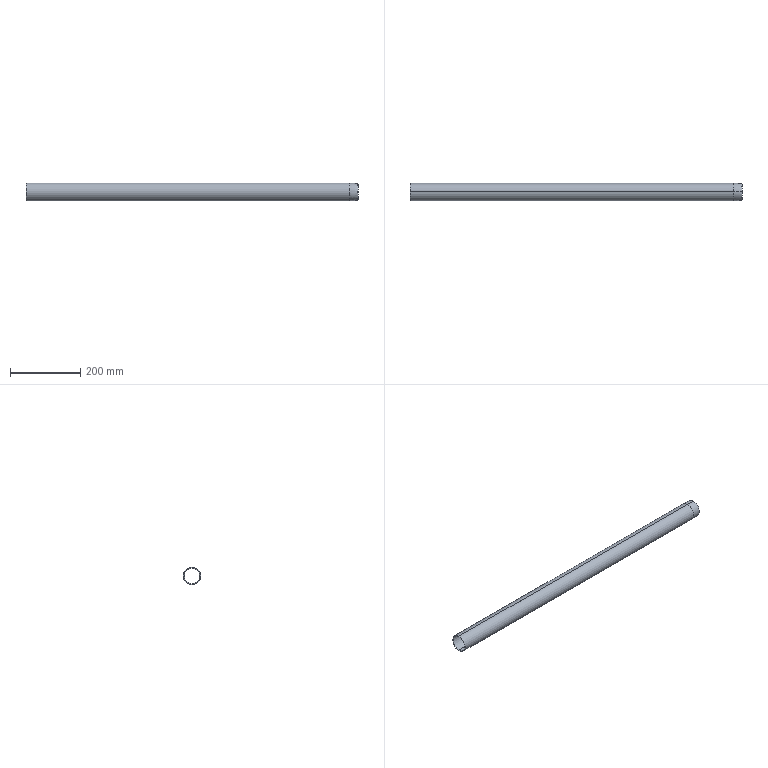Part | SolidWorks | features BaseBody 1 | 1 solid | 12 faces | box 947.5 x 50 x 50 mm | volume 174207 mm3 | torus 6 | cylinder 4 | plane 2 | commonest cylinder face diameters 47.6 x2 50 x2
STEP:
#1=CARTESIAN_POINT('',(922.5,0.,-23.8));
#2=VERTEX_POINT('',#1);
#3=CARTESIAN_POINT('',(922.5,0.,23.8));
#4=VERTEX_POINT('',#3);
#5=CARTESIAN_POINT('',(922.5,0.,0.));
#6=DIRECTION('',(-1.,0.,0.));
#7=DIRECTION('',(0.,0.,1.));
#8=AXIS2_PLACEMENT_3D('',#5,#6,#7);
#9=CIRCLE('',#8,23.8);
#10=EDGE_CURVE('',#2,#4,#9,.T.);
#11=ORIENTED_EDGE('',*,*,#10,.F.);
#12=CARTESIAN_POINT('',(0.,0.,-23.8));
#13=VERTEX_POINT('',#12);
#14=CARTESIAN_POINT('',(0.,0.,-23.8));
#15=DIRECTION('',(-1.,0.,0.));
#16=VECTOR('',#15,1000.);
#17=LINE('',#14,#16);
#18=EDGE_CURVE('',#2,#13,#17,.T.);
#19=ORIENTED_EDGE('',*,*,#18,.T.);
#20=CARTESIAN_POINT('',(0.,0.,23.8));
#21=VERTEX_POINT('',#20);
#22=CARTESIAN_POINT('',(0.,0.,0.));
#23=DIRECTION('',(-1.,0.,0.));
#24=DIRECTION('',(0.,0.,-1.));
#25=AXIS2_PLACEMENT_3D('',#22,#23,#24);
#26=CIRCLE('',#25,23.8);
#27=EDGE_CURVE('',#13,#21,#26,.T.);
#28=ORIENTED_EDGE('',*,*,#27,.T.);
#29=CARTESIAN_POINT('',(0.,0.,23.8));
#30=DIRECTION('',(-1.,0.,0.));
#31=VECTOR('',#30,1000.);
#32=LINE('',#29,#31);
#33=EDGE_CURVE('',#4,#21,#32,.T.);
#34=ORIENTED_EDGE('',*,*,#33,.F.);
#35=EDGE_LOOP('',(#11,#19,#28,#34));
#36=FACE_OUTER_BOUND('',#35,.T.);
#37=CARTESIAN_POINT('',(0.,0.,0.));
#38=DIRECTION('',(-1.,0.,0.));
#39=DIRECTION('',(0.,0.,1.));
#40=AXIS2_PLACEMENT_3D('',#37,#38,#39);
#41=CYLINDRICAL_SURFACE('',#40,23.8);
#42=ADVANCED_FACE('',(#36),#41,.F.);
#43=CARTESIAN_POINT('',(947.5,0.,-21.938));
#44=VERTEX_POINT('',#43);
#45=CARTESIAN_POINT('',(947.5,0.,21.938));
#46=VERTEX_POINT('',#45);
#47=CARTESIAN_POINT('',(947.5,0.,0.));
#48=DIRECTION('',(-1.,0.,0.));
#49=DIRECTION('',(0.,0.,1.));
#50=AXIS2_PLACEMENT_3D('',#47,#48,#49);
#51=CIRCLE('',#50,21.938);
#52=EDGE_CURVE('',#44,#46,#51,.T.);
#53=ORIENTED_EDGE('',*,*,#52,.F.);
#54=CARTESIAN_POINT('',(922.5,0.,145.));
#55=DIRECTION('',(0.,1.,0.));
#56=DIRECTION('',(0.,0.,1.));
#57=AXIS2_PLACEMENT_3D('',#54,#55,#56);
#58=CIRCLE('',#57,168.8);
#59=EDGE_CURVE('',#44,#2,#58,.T.);
#60=ORIENTED_EDGE('',*,*,#59,.T.);
#61=ORIENTED_EDGE('',*,*,#10,.T.);
#62=CARTESIAN_POINT('',(922.5,0.,-145.));
#63=DIRECTION('',(0.,-1.,0.));
#64=DIRECTION('',(0.,0.,-1.));
#65=AXIS2_PLACEMENT_3D('',#62,#63,#64);
#66=CIRCLE('',#65,168.8);
#67=EDGE_CURVE('',#46,#4,#66,.T.);
#68=ORIENTED_EDGE('',*,*,#67,.F.);
#69=EDGE_LOOP('',(#53,#60,#61,#68));
#70=FACE_OUTER_BOUND('',#69,.T.);
#71=CARTESIAN_POINT('',(922.5,0.,0.));
#72=DIRECTION('',(-1.,0.,0.));
#73=DIRECTION('',(0.,0.,1.));
#74=AXIS2_PLACEMENT_3D('',#71,#72,#73);
#75=TOROIDAL_SURFACE('',#74,-145.,168.8);
#76=ADVANCED_FACE('',(#70),#75,.F.);
#77=CARTESIAN_POINT('',(922.5,0.,25.));
#78=VERTEX_POINT('',#77);
#79=CARTESIAN_POINT('',(922.5,0.,-25.));
#80=VERTEX_POINT('',#79);
#81=CARTESIAN_POINT('',(922.5,0.,0.));
#82=DIRECTION('',(-1.,0.,0.));
#83=DIRECTION('',(0.,0.,1.));
#84=AXIS2_PLACEMENT_3D('',#81,#82,#83);
#85=CIRCLE('',#84,25.);
#86=EDGE_CURVE('',#78,#80,#85,.T.);
#87=ORIENTED_EDGE('',*,*,#86,.T.);
#88=CARTESIAN_POINT('',(0.,0.,-25.));
#89=VERTEX_POINT('',#88);
#90=CARTESIAN_POINT('',(0.,0.,-25.));
#91=DIRECTION('',(-1.,0.,0.));
#92=VECTOR('',#91,1000.);
#93=LINE('',#90,#92);
#94=EDGE_CURVE('',#80,#89,#93,.T.);
#95=ORIENTED_EDGE('',*,*,#94,.T.);
#96=CARTESIAN_POINT('',(0.,0.,25.));
#97=VERTEX_POINT('',#96);
#98=CARTESIAN_POINT('',(0.,0.,0.));
#99=DIRECTION('',(-1.,0.,0.));
#100=DIRECTION('',(0.,0.,1.));
#101=AXIS2_PLACEMENT_3D('',#98,#99,#100);
#102=CIRCLE('',#101,25.);
#103=EDGE_CURVE('',#97,#89,#102,.T.);
#104=ORIENTED_EDGE('',*,*,#103,.F.);
#105=CARTESIAN_POINT('',(0.,0.,25.));
#106=DIRECTION('',(-1.,0.,0.));
#107=VECTOR('',#106,1000.);
#108=LINE('',#105,#107);
#109=EDGE_CURVE('',#78,#97,#108,.T.);
#110=ORIENTED_EDGE('',*,*,#109,.F.);
#111=EDGE_LOOP('',(#87,#95,#104,#110));
#112=FACE_OUTER_BOUND('',#111,.T.);
#113=CARTESIAN_POINT('',(0.,0.,0.));
#114=DIRECTION('',(-1.,0.,0.));
#115=DIRECTION('',(0.,0.,1.));
#116=AXIS2_PLACEMENT_3D('',#113,#114,#115);
#117=CYLINDRICAL_SURFACE('',#116,25.);
#118=ADVANCED_FACE('',(#112),#117,.T.);
#119=CARTESIAN_POINT('',(947.072,0.,23.215));
#120=VERTEX_POINT('',#119);
#121=CARTESIAN_POINT('',(947.072,0.,-23.215));
#122=VERTEX_POINT('',#121);
#123=CARTESIAN_POINT('',(947.072,0.,0.));
#124=DIRECTION('',(-1.,0.,0.));
#125=DIRECTION('',(0.,0.,1.));
#126=AXIS2_PLACEMENT_3D('',#123,#124,#125);
#127=CIRCLE('',#126,23.215);
#128=EDGE_CURVE('',#120,#122,#127,.T.);
#129=ORIENTED_EDGE('',*,*,#128,.T.);
#130=CARTESIAN_POINT('',(922.5,0.,145.));
#131=DIRECTION('',(0.,1.,0.));
#132=DIRECTION('',(0.,0.,1.));
#133=AXIS2_PLACEMENT_3D('',#130,#131,#132);
#134=CIRCLE('',#133,170.);
#135=EDGE_CURVE('',#122,#80,#134,.T.);
#136=ORIENTED_EDGE('',*,*,#135,.T.);
#137=ORIENTED_EDGE('',*,*,#86,.F.);
#138=CARTESIAN_POINT('',(922.5,0.,-145.));
#139=DIRECTION('',(0.,-1.,0.));
#140=DIRECTION('',(0.,0.,-1.));
#141=AXIS2_PLACEMENT_3D('',#138,#139,#140);
#142=CIRCLE('',#141,170.);
#143=EDGE_CURVE('',#120,#78,#142,.T.);
#144=ORIENTED_EDGE('',*,*,#143,.F.);
#145=EDGE_LOOP('',(#129,#136,#137,#144));
#146=FACE_OUTER_BOUND('',#145,.T.);
#147=CARTESIAN_POINT('',(922.5,0.,0.));
#148=DIRECTION('',(-1.,0.,0.));
#149=DIRECTION('',(0.,0.,1.));
#150=AXIS2_PLACEMENT_3D('',#147,#148,#149);
#151=TOROIDAL_SURFACE('',#150,-145.,170.);
#152=ADVANCED_FACE('',(#146),#151,.T.);
#153=CARTESIAN_POINT('',(947.5,0.,22.72));
#154=VERTEX_POINT('',#153);
#155=CARTESIAN_POINT('',(947.5,0.,-22.72));
#156=VERTEX_POINT('',#155);
#157=CARTESIAN_POINT('',(947.5,0.,0.));
#158=DIRECTION('',(-1.,0.,0.));
#159=DIRECTION('',(0.,0.,1.));
#160=AXIS2_PLACEMENT_3D('',#157,#158,#159);
#161=CIRCLE('',#160,22.72);
#162=EDGE_CURVE('',#154,#156,#161,.T.);
#163=ORIENTED_EDGE('',*,*,#162,.T.);
#164=CARTESIAN_POINT('',(947.,0.,-22.72));
#165=DIRECTION('',(0.,1.,0.));
#166=DIRECTION('',(0.,0.,1.));
#167=AXIS2_PLACEMENT_3D('',#164,#165,#166);
#168=CIRCLE('',#167,0.5);
#169=EDGE_CURVE('',#156,#122,#168,.T.);
#170=ORIENTED_EDGE('',*,*,#169,.T.);
#171=ORIENTED_EDGE('',*,*,#128,.F.);
#172=CARTESIAN_POINT('',(947.,0.,22.72));
#173=DIRECTION('',(0.,-1.,0.));
#174=DIRECTION('',(0.,0.,-1.));
#175=AXIS2_PLACEMENT_3D('',#172,#173,#174);
#176=CIRCLE('',#175,0.5);
#177=EDGE_CURVE('',#154,#120,#176,.T.);
#178=ORIENTED_EDGE('',*,*,#177,.F.);
#179=EDGE_LOOP('',(#163,#170,#171,#178));
#180=FACE_OUTER_BOUND('',#179,.T.);
#181=CARTESIAN_POINT('',(947.,0.,0.));
#182=DIRECTION('',(-1.,0.,0.));
#183=DIRECTION('',(0.,0.,1.));
#184=AXIS2_PLACEMENT_3D('',#181,#182,#183);
#185=TOROIDAL_SURFACE('',#184,22.72,0.5);
#186=ADVANCED_FACE('',(#180),#185,.T.);
#187=CARTESIAN_POINT('',(947.5,0.,0.));
#188=DIRECTION('',(-1.,0.,0.));
#189=DIRECTION('',(0.,0.,1.));
#190=AXIS2_PLACEMENT_3D('',#187,#188,#189);
#191=CIRCLE('',#190,21.938);
#192=EDGE_CURVE('',#46,#44,#191,.T.);
#193=ORIENTED_EDGE('',*,*,#192,.T.);
#194=ORIENTED_EDGE('',*,*,#52,.T.);
#195=EDGE_LOOP('',(#193,#194));
#196=FACE_BOUND('',#195,.T.);
#197=ORIENTED_EDGE('',*,*,#162,.F.);
#198=CARTESIAN_POINT('',(947.5,0.,0.));
#199=DIRECTION('',(-1.,0.,0.));
#200=DIRECTION('',(0.,0.,1.));
#201=AXIS2_PLACEMENT_3D('',#198,#199,#200);
#202=CIRCLE('',#201,22.72);
#203=EDGE_CURVE('',#156,#154,#202,.T.);
#204=ORIENTED_EDGE('',*,*,#203,.F.);
#205=EDGE_LOOP('',(#197,#204));
#206=FACE_OUTER_BOUND('',#205,.T.);
#207=CARTESIAN_POINT('',(947.5,22.72,0.));
#208=DIRECTION('',(-1.,0.,0.));
#209=DIRECTION('',(0.,0.,1.));
#210=AXIS2_PLACEMENT_3D('',#207,#208,#209);
#211=PLANE('',#210);
#212=ADVANCED_FACE('',(#196,#206),#211,.F.);
#213=ORIENTED_EDGE('',*,*,#169,.F.);
#214=ORIENTED_EDGE('',*,*,#203,.T.);
#215=ORIENTED_EDGE('',*,*,#177,.T.);
#216=CARTESIAN_POINT('',(947.072,0.,0.));
#217=DIRECTION('',(-1.,0.,0.));
#218=DIRECTION('',(0.,0.,1.));
#219=AXIS2_PLACEMENT_3D('',#216,#217,#218);
#220=CIRCLE('',#219,23.215);
#221=EDGE_CURVE('',#122,#120,#220,.T.);
#222=ORIENTED_EDGE('',*,*,#221,.F.);
#223=EDGE_LOOP('',(#213,#214,#215,#222));
#224=FACE_OUTER_BOUND('',#223,.T.);
#225=CARTESIAN_POINT('',(947.,0.,0.));
#226=DIRECTION('',(-1.,0.,0.));
#227=DIRECTION('',(0.,0.,1.));
#228=AXIS2_PLACEMENT_3D('',#225,#226,#227);
#229=TOROIDAL_SURFACE('',#228,22.72,0.5);
#230=ADVANCED_FACE('',(#224),#229,.T.);
#231=ORIENTED_EDGE('',*,*,#135,.F.);
#232=ORIENTED_EDGE('',*,*,#221,.T.);
#233=ORIENTED_EDGE('',*,*,#143,.T.);
#234=CARTESIAN_POINT('',(922.5,0.,0.));
#235=DIRECTION('',(-1.,0.,0.));
#236=DIRECTION('',(0.,0.,1.));
#237=AXIS2_PLACEMENT_3D('',#234,#235,#236);
#238=CIRCLE('',#237,25.);
#239=EDGE_CURVE('',#80,#78,#238,.T.);
#240=ORIENTED_EDGE('',*,*,#239,.F.);
#241=EDGE_LOOP('',(#231,#232,#233,#240));
#242=FACE_OUTER_BOUND('',#241,.T.);
#243=CARTESIAN_POINT('',(922.5,0.,0.));
#244=DIRECTION('',(-1.,0.,0.));
#245=DIRECTION('',(0.,0.,1.));
#246=AXIS2_PLACEMENT_3D('',#243,#244,#245);
#247=TOROIDAL_SURFACE('',#246,-145.,170.);
#248=ADVANCED_FACE('',(#242),#247,.T.);
#249=ORIENTED_EDGE('',*,*,#94,.F.);
#250=ORIENTED_EDGE('',*,*,#239,.T.);
#251=ORIENTED_EDGE('',*,*,#109,.T.);
#252=CARTESIAN_POINT('',(0.,0.,0.));
#253=DIRECTION('',(-1.,0.,0.));
#254=DIRECTION('',(0.,0.,1.));
#255=AXIS2_PLACEMENT_3D('',#252,#253,#254);
#256=CIRCLE('',#255,25.);
#257=EDGE_CURVE('',#89,#97,#256,.T.);
#258=ORIENTED_EDGE('',*,*,#257,.F.);
#259=EDGE_LOOP('',(#249,#250,#251,#258));
#260=FACE_OUTER_BOUND('',#259,.T.);
#261=CARTESIAN_POINT('',(0.,0.,0.));
#262=DIRECTION('',(-1.,0.,0.));
#263=DIRECTION('',(0.,0.,1.));
#264=AXIS2_PLACEMENT_3D('',#261,#262,#263);
#265=CYLINDRICAL_SURFACE('',#264,25.);
#266=ADVANCED_FACE('',(#260),#265,.T.);
#267=CARTESIAN_POINT('',(0.,0.,0.));
#268=DIRECTION('',(-1.,0.,0.));
#269=DIRECTION('',(0.,0.,-1.));
#270=AXIS2_PLACEMENT_3D('',#267,#268,#269);
#271=CIRCLE('',#270,23.8);
#272=EDGE_CURVE('',#21,#13,#271,.T.);
#273=ORIENTED_EDGE('',*,*,#272,.F.);
#274=ORIENTED_EDGE('',*,*,#27,.F.);
#275=EDGE_LOOP('',(#273,#274));
#276=FACE_BOUND('',#275,.T.);
#277=ORIENTED_EDGE('',*,*,#103,.T.);
#278=ORIENTED_EDGE('',*,*,#257,.T.);
#279=EDGE_LOOP('',(#277,#278));
#280=FACE_OUTER_BOUND('',#279,.T.);
#281=CARTESIAN_POINT('',(0.,0.,0.));
#282=DIRECTION('',(1.,0.,0.));
#283=DIRECTION('',(0.,0.,-1.));
#284=AXIS2_PLACEMENT_3D('',#281,#282,#283);
#285=PLANE('',#284);
#286=ADVANCED_FACE('',(#276,#280),#285,.F.);
#287=ORIENTED_EDGE('',*,*,#59,.F.);
#288=ORIENTED_EDGE('',*,*,#192,.F.);
#289=ORIENTED_EDGE('',*,*,#67,.T.);
#290=CARTESIAN_POINT('',(922.5,0.,0.));
#291=DIRECTION('',(-1.,0.,0.));
#292=DIRECTION('',(0.,0.,1.));
#293=AXIS2_PLACEMENT_3D('',#290,#291,#292);
#294=CIRCLE('',#293,23.8);
#295=EDGE_CURVE('',#4,#2,#294,.T.);
#296=ORIENTED_EDGE('',*,*,#295,.T.);
#297=EDGE_LOOP('',(#287,#288,#289,#296));
#298=FACE_OUTER_BOUND('',#297,.T.);
#299=CARTESIAN_POINT('',(922.5,0.,0.));
#300=DIRECTION('',(-1.,0.,0.));
#301=DIRECTION('',(0.,0.,1.));
#302=AXIS2_PLACEMENT_3D('',#299,#300,#301);
#303=TOROIDAL_SURFACE('',#302,-145.,168.8);
#304=ADVANCED_FACE('',(#298),#303,.F.);
#305=ORIENTED_EDGE('',*,*,#18,.F.);
#306=ORIENTED_EDGE('',*,*,#295,.F.);
#307=ORIENTED_EDGE('',*,*,#33,.T.);
#308=ORIENTED_EDGE('',*,*,#272,.T.);
#309=EDGE_LOOP('',(#305,#306,#307,#308));
#310=FACE_OUTER_BOUND('',#309,.T.);
#311=CARTESIAN_POINT('',(0.,0.,0.));
#312=DIRECTION('',(-1.,0.,0.));
#313=DIRECTION('',(0.,0.,1.));
#314=AXIS2_PLACEMENT_3D('',#311,#312,#313);
#315=CYLINDRICAL_SURFACE('',#314,23.8);
#316=ADVANCED_FACE('',(#310),#315,.F.);
#317=CLOSED_SHELL('',(#42,#76,#118,#152,#186,#212,#230,#248,#266,#286,#304,#316));
#318=MANIFOLD_SOLID_BREP('',#317);
#319=CARTESIAN_POINT('',(0.,0.,0.));
#320=DIRECTION('',(0.,0.,1.));
#321=DIRECTION('',(1.,0.,0.));
#322=AXIS2_PLACEMENT_3D('',#319,#320,#321);
#323=(LENGTH_UNIT()NAMED_UNIT(*)SI_UNIT(.MILLI.,.METRE.));
#324=UNCERTAINTY_MEASURE_WITH_UNIT(LENGTH_MEASURE(0.00001),#323,'','');
#325=(NAMED_UNIT(*)PLANE_ANGLE_UNIT()SI_UNIT($,.RADIAN.));
#326=(NAMED_UNIT(*)SI_UNIT($,.STERADIAN.)SOLID_ANGLE_UNIT());
#327=(GEOMETRIC_REPRESENTATION_CONTEXT(3)GLOBAL_UNCERTAINTY_ASSIGNED_CONTEXT((#324))GLOBAL_UNIT_ASSIGNED_CONTEXT((#323,#325,#326))REPRESENTATION_CONTEXT('',''));
#328=ADVANCED_BREP_SHAPE_REPRESENTATION('',(#318,#322),#327);